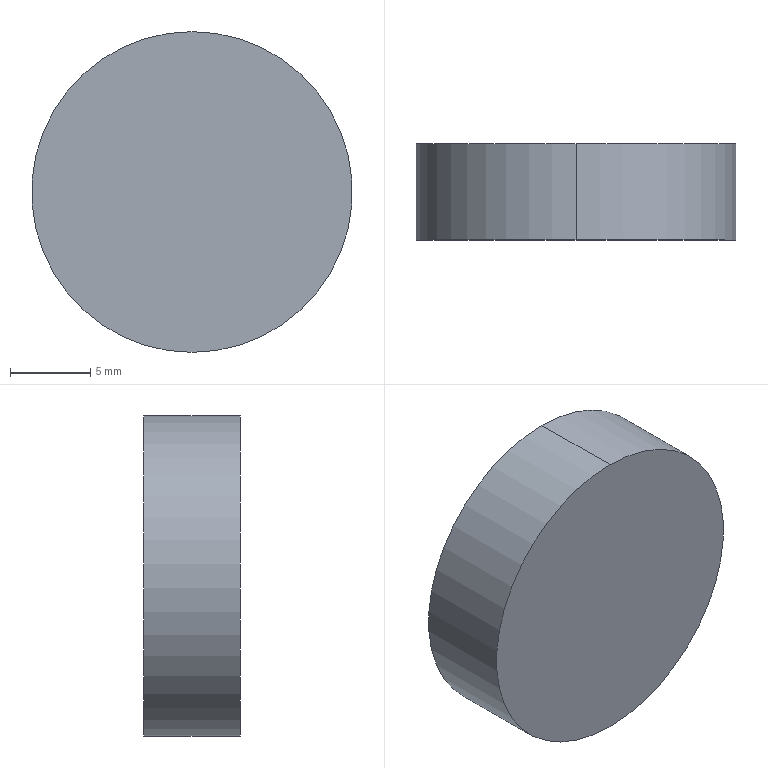Part | SolidWorks | features Extrusion 1 | 1 solid | 4 faces | box 20 x 6 x 20 mm | volume 1885 mm3 | cylinder 2 | plane 2 | commonest cylinder face diameters 20 x2
STEP:
#1=CARTESIAN_POINT('',(0.,6.,10.));
#2=VERTEX_POINT('',#1);
#3=CARTESIAN_POINT('',(0.,6.,-10.));
#4=VERTEX_POINT('',#3);
#5=CARTESIAN_POINT('',(0.,6.,0.));
#6=DIRECTION('',(0.,1.,0.));
#7=DIRECTION('',(0.,0.,1.));
#8=AXIS2_PLACEMENT_3D('',#5,#6,#7);
#9=CIRCLE('',#8,10.);
#10=EDGE_CURVE('',#2,#4,#9,.T.);
#11=ORIENTED_EDGE('',*,*,#10,.F.);
#12=CARTESIAN_POINT('',(0.,0.,10.));
#13=VERTEX_POINT('',#12);
#14=CARTESIAN_POINT('',(0.,6.,10.));
#15=DIRECTION('',(0.,-1.,0.));
#16=VECTOR('',#15,1000.);
#17=LINE('',#14,#16);
#18=EDGE_CURVE('',#2,#13,#17,.T.);
#19=ORIENTED_EDGE('',*,*,#18,.T.);
#20=CARTESIAN_POINT('',(0.,0.,-10.));
#21=VERTEX_POINT('',#20);
#22=CARTESIAN_POINT('',(0.,0.,0.));
#23=DIRECTION('',(0.,1.,0.));
#24=DIRECTION('',(0.,0.,1.));
#25=AXIS2_PLACEMENT_3D('',#22,#23,#24);
#26=CIRCLE('',#25,10.);
#27=EDGE_CURVE('',#13,#21,#26,.T.);
#28=ORIENTED_EDGE('',*,*,#27,.T.);
#29=CARTESIAN_POINT('',(0.,6.,-10.));
#30=DIRECTION('',(0.,-1.,0.));
#31=VECTOR('',#30,1000.);
#32=LINE('',#29,#31);
#33=EDGE_CURVE('',#4,#21,#32,.T.);
#34=ORIENTED_EDGE('',*,*,#33,.F.);
#35=EDGE_LOOP('',(#11,#19,#28,#34));
#36=FACE_OUTER_BOUND('',#35,.T.);
#37=CARTESIAN_POINT('',(0.,6.,0.));
#38=DIRECTION('',(0.,-1.,0.));
#39=DIRECTION('',(0.,0.,-1.));
#40=AXIS2_PLACEMENT_3D('',#37,#38,#39);
#41=CYLINDRICAL_SURFACE('',#40,10.);
#42=ADVANCED_FACE('',(#36),#41,.T.);
#43=ORIENTED_EDGE('',*,*,#18,.F.);
#44=CARTESIAN_POINT('',(0.,6.,0.));
#45=DIRECTION('',(0.,1.,0.));
#46=DIRECTION('',(0.,0.,1.));
#47=AXIS2_PLACEMENT_3D('',#44,#45,#46);
#48=CIRCLE('',#47,10.);
#49=EDGE_CURVE('',#4,#2,#48,.T.);
#50=ORIENTED_EDGE('',*,*,#49,.F.);
#51=ORIENTED_EDGE('',*,*,#33,.T.);
#52=CARTESIAN_POINT('',(0.,0.,0.));
#53=DIRECTION('',(0.,1.,0.));
#54=DIRECTION('',(0.,0.,1.));
#55=AXIS2_PLACEMENT_3D('',#52,#53,#54);
#56=CIRCLE('',#55,10.);
#57=EDGE_CURVE('',#21,#13,#56,.T.);
#58=ORIENTED_EDGE('',*,*,#57,.T.);
#59=EDGE_LOOP('',(#43,#50,#51,#58));
#60=FACE_OUTER_BOUND('',#59,.T.);
#61=CARTESIAN_POINT('',(0.,6.,0.));
#62=DIRECTION('',(0.,-1.,0.));
#63=DIRECTION('',(0.,0.,-1.));
#64=AXIS2_PLACEMENT_3D('',#61,#62,#63);
#65=CYLINDRICAL_SURFACE('',#64,10.);
#66=ADVANCED_FACE('',(#60),#65,.T.);
#67=ORIENTED_EDGE('',*,*,#49,.T.);
#68=ORIENTED_EDGE('',*,*,#10,.T.);
#69=EDGE_LOOP('',(#67,#68));
#70=FACE_OUTER_BOUND('',#69,.T.);
#71=CARTESIAN_POINT('',(0.,6.,0.));
#72=DIRECTION('',(0.,1.,0.));
#73=DIRECTION('',(0.,0.,1.));
#74=AXIS2_PLACEMENT_3D('',#71,#72,#73);
#75=PLANE('',#74);
#76=ADVANCED_FACE('',(#70),#75,.T.);
#77=ORIENTED_EDGE('',*,*,#57,.F.);
#78=ORIENTED_EDGE('',*,*,#27,.F.);
#79=EDGE_LOOP('',(#77,#78));
#80=FACE_OUTER_BOUND('',#79,.T.);
#81=CARTESIAN_POINT('',(0.,0.,0.));
#82=DIRECTION('',(0.,1.,0.));
#83=DIRECTION('',(0.,0.,1.));
#84=AXIS2_PLACEMENT_3D('',#81,#82,#83);
#85=PLANE('',#84);
#86=ADVANCED_FACE('',(#80),#85,.F.);
#87=CLOSED_SHELL('',(#42,#66,#76,#86));
#88=MANIFOLD_SOLID_BREP('',#87);
#89=CARTESIAN_POINT('',(0.,0.,0.));
#90=DIRECTION('',(0.,0.,1.));
#91=DIRECTION('',(1.,0.,0.));
#92=AXIS2_PLACEMENT_3D('',#89,#90,#91);
#93=(LENGTH_UNIT()NAMED_UNIT(*)SI_UNIT(.MILLI.,.METRE.));
#94=UNCERTAINTY_MEASURE_WITH_UNIT(LENGTH_MEASURE(0.00001),#93,'','');
#95=(NAMED_UNIT(*)PLANE_ANGLE_UNIT()SI_UNIT($,.RADIAN.));
#96=(NAMED_UNIT(*)SI_UNIT($,.STERADIAN.)SOLID_ANGLE_UNIT());
#97=(GEOMETRIC_REPRESENTATION_CONTEXT(3)GLOBAL_UNCERTAINTY_ASSIGNED_CONTEXT((#94))GLOBAL_UNIT_ASSIGNED_CONTEXT((#93,#95,#96))REPRESENTATION_CONTEXT('',''));
#98=ADVANCED_BREP_SHAPE_REPRESENTATION('',(#88,#92),#97);